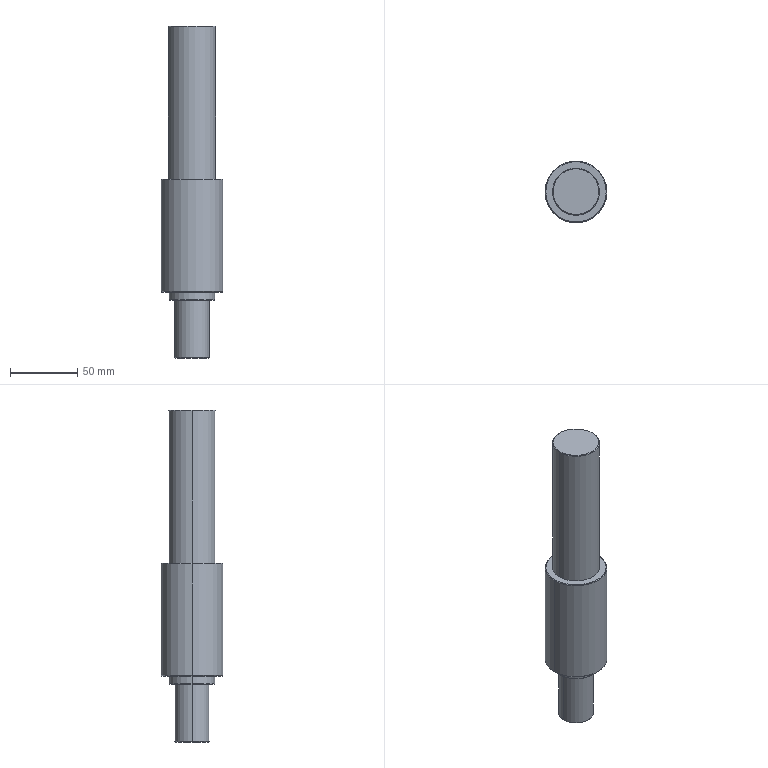Part | SolidWorks | features ICE 3, Chamfer 1, Extrusion 1 | 1 solid | 23 faces | box 46 x 46 x 247 mm | volume 277485 mm3 | cone 10 | cylinder 8 | plane 5 | commonest cylinder face diameters 26 x2 34 x2 35 x2 46 x2
STEP:
#1=CARTESIAN_POINT('',(17.,0.,57.));
#2=VERTEX_POINT('',#1);
#3=CARTESIAN_POINT('',(-17.,0.,57.));
#4=VERTEX_POINT('',#3);
#5=CARTESIAN_POINT('',(0.,0.,57.));
#6=DIRECTION('',(0.,0.,1.));
#7=DIRECTION('',(1.,0.,0.));
#8=AXIS2_PLACEMENT_3D('',#5,#6,#7);
#9=CIRCLE('',#8,17.);
#10=EDGE_CURVE('',#2,#4,#9,.T.);
#11=ORIENTED_EDGE('',*,*,#10,.F.);
#12=CARTESIAN_POINT('',(17.5,0.,56.5));
#13=VERTEX_POINT('',#12);
#14=CARTESIAN_POINT('',(17.,0.,57.));
#15=DIRECTION('',(0.7071,0.,-0.7071));
#16=VECTOR('',#15,1000.);
#17=LINE('',#14,#16);
#18=EDGE_CURVE('',#2,#13,#17,.T.);
#19=ORIENTED_EDGE('',*,*,#18,.T.);
#20=CARTESIAN_POINT('',(-17.5,0.,56.5));
#21=VERTEX_POINT('',#20);
#22=CARTESIAN_POINT('',(0.,0.,56.5));
#23=DIRECTION('',(0.,0.,-1.));
#24=DIRECTION('',(1.,0.,0.));
#25=AXIS2_PLACEMENT_3D('',#22,#23,#24);
#26=CIRCLE('',#25,17.5);
#27=EDGE_CURVE('',#21,#13,#26,.T.);
#28=ORIENTED_EDGE('',*,*,#27,.F.);
#29=CARTESIAN_POINT('',(-17.,0.,57.));
#30=DIRECTION('',(-0.7071,0.,-0.7071));
#31=VECTOR('',#30,1000.);
#32=LINE('',#29,#31);
#33=EDGE_CURVE('',#4,#21,#32,.T.);
#34=ORIENTED_EDGE('',*,*,#33,.F.);
#35=EDGE_LOOP('',(#11,#19,#28,#34));
#36=FACE_OUTER_BOUND('',#35,.T.);
#37=CARTESIAN_POINT('',(0.,0.,57.));
#38=DIRECTION('',(0.,0.,-1.));
#39=DIRECTION('',(-1.,0.,0.));
#40=AXIS2_PLACEMENT_3D('',#37,#38,#39);
#41=CONICAL_SURFACE('',#40,17.,0.7854);
#42=ADVANCED_FACE('',(#36),#41,.T.);
#43=CARTESIAN_POINT('',(22.5,0.,-57.));
#44=VERTEX_POINT('',#43);
#45=CARTESIAN_POINT('',(-22.5,0.,-57.));
#46=VERTEX_POINT('',#45);
#47=CARTESIAN_POINT('',(0.,0.,-57.));
#48=DIRECTION('',(0.,0.,1.));
#49=DIRECTION('',(-1.,0.,0.));
#50=AXIS2_PLACEMENT_3D('',#47,#48,#49);
#51=CIRCLE('',#50,22.5);
#52=EDGE_CURVE('',#44,#46,#51,.T.);
#53=ORIENTED_EDGE('',*,*,#52,.F.);
#54=CARTESIAN_POINT('',(23.,0.,-57.5));
#55=VERTEX_POINT('',#54);
#56=CARTESIAN_POINT('',(23.,0.,-57.5));
#57=DIRECTION('',(0.7071,0.,-0.7071));
#58=VECTOR('',#57,1000.);
#59=LINE('',#56,#58);
#60=EDGE_CURVE('',#44,#55,#59,.T.);
#61=ORIENTED_EDGE('',*,*,#60,.T.);
#62=CARTESIAN_POINT('',(-23.,0.,-57.5));
#63=VERTEX_POINT('',#62);
#64=CARTESIAN_POINT('',(0.,0.,-57.5));
#65=DIRECTION('',(0.,0.,-1.));
#66=DIRECTION('',(-1.,0.,0.));
#67=AXIS2_PLACEMENT_3D('',#64,#65,#66);
#68=CIRCLE('',#67,23.);
#69=EDGE_CURVE('',#63,#55,#68,.T.);
#70=ORIENTED_EDGE('',*,*,#69,.F.);
#71=CARTESIAN_POINT('',(-23.,0.,-57.5));
#72=DIRECTION('',(-0.7071,0.,-0.7071));
#73=VECTOR('',#72,1000.);
#74=LINE('',#71,#73);
#75=EDGE_CURVE('',#46,#63,#74,.T.);
#76=ORIENTED_EDGE('',*,*,#75,.F.);
#77=EDGE_LOOP('',(#53,#61,#70,#76));
#78=FACE_OUTER_BOUND('',#77,.T.);
#79=CARTESIAN_POINT('',(0.,0.,-57.5));
#80=DIRECTION('',(0.,0.,-1.));
#81=DIRECTION('',(-1.,0.,0.));
#82=AXIS2_PLACEMENT_3D('',#79,#80,#81);
#83=CONICAL_SURFACE('',#82,23.,0.7854);
#84=ADVANCED_FACE('',(#78),#83,.T.);
#85=CARTESIAN_POINT('',(-16.5,0.,-147.));
#86=VERTEX_POINT('',#85);
#87=CARTESIAN_POINT('',(16.5,0.,-147.));
#88=VERTEX_POINT('',#87);
#89=CARTESIAN_POINT('',(0.,0.,-147.));
#90=DIRECTION('',(0.,0.,-1.));
#91=DIRECTION('',(-1.,0.,0.));
#92=AXIS2_PLACEMENT_3D('',#89,#90,#91);
#93=CIRCLE('',#92,16.5);
#94=EDGE_CURVE('',#86,#88,#93,.T.);
#95=ORIENTED_EDGE('',*,*,#94,.F.);
#96=CARTESIAN_POINT('',(-17.,0.,-146.5));
#97=VERTEX_POINT('',#96);
#98=CARTESIAN_POINT('',(-16.5,0.,-147.));
#99=DIRECTION('',(-0.7071,0.,0.7071));
#100=VECTOR('',#99,1000.);
#101=LINE('',#98,#100);
#102=EDGE_CURVE('',#86,#97,#101,.T.);
#103=ORIENTED_EDGE('',*,*,#102,.T.);
#104=CARTESIAN_POINT('',(17.,0.,-146.5));
#105=VERTEX_POINT('',#104);
#106=CARTESIAN_POINT('',(0.,0.,-146.5));
#107=DIRECTION('',(0.,0.,1.));
#108=DIRECTION('',(-1.,0.,0.));
#109=AXIS2_PLACEMENT_3D('',#106,#107,#108);
#110=CIRCLE('',#109,17.);
#111=EDGE_CURVE('',#105,#97,#110,.T.);
#112=ORIENTED_EDGE('',*,*,#111,.F.);
#113=CARTESIAN_POINT('',(16.5,0.,-147.));
#114=DIRECTION('',(0.7071,0.,0.7071));
#115=VECTOR('',#114,1000.);
#116=LINE('',#113,#115);
#117=EDGE_CURVE('',#88,#105,#116,.T.);
#118=ORIENTED_EDGE('',*,*,#117,.F.);
#119=EDGE_LOOP('',(#95,#103,#112,#118));
#120=FACE_OUTER_BOUND('',#119,.T.);
#121=CARTESIAN_POINT('',(0.,0.,-147.));
#122=DIRECTION('',(0.,0.,1.));
#123=DIRECTION('',(1.,0.,0.));
#124=AXIS2_PLACEMENT_3D('',#121,#122,#123);
#125=CONICAL_SURFACE('',#124,16.5,0.7854);
#126=ADVANCED_FACE('',(#120),#125,.T.);
#127=CARTESIAN_POINT('',(-22.5,0.,-141.));
#128=VERTEX_POINT('',#127);
#129=CARTESIAN_POINT('',(22.5,0.,-141.));
#130=VERTEX_POINT('',#129);
#131=CARTESIAN_POINT('',(0.,0.,-141.));
#132=DIRECTION('',(0.,0.,-1.));
#133=DIRECTION('',(-1.,0.,0.));
#134=AXIS2_PLACEMENT_3D('',#131,#132,#133);
#135=CIRCLE('',#134,22.5);
#136=EDGE_CURVE('',#128,#130,#135,.T.);
#137=ORIENTED_EDGE('',*,*,#136,.F.);
#138=CARTESIAN_POINT('',(-23.,0.,-140.5));
#139=VERTEX_POINT('',#138);
#140=CARTESIAN_POINT('',(-22.5,0.,-141.));
#141=DIRECTION('',(-0.7071,0.,0.7071));
#142=VECTOR('',#141,1000.);
#143=LINE('',#140,#142);
#144=EDGE_CURVE('',#128,#139,#143,.T.);
#145=ORIENTED_EDGE('',*,*,#144,.T.);
#146=CARTESIAN_POINT('',(23.,0.,-140.5));
#147=VERTEX_POINT('',#146);
#148=CARTESIAN_POINT('',(0.,0.,-140.5));
#149=DIRECTION('',(0.,0.,1.));
#150=DIRECTION('',(-1.,0.,0.));
#151=AXIS2_PLACEMENT_3D('',#148,#149,#150);
#152=CIRCLE('',#151,23.);
#153=EDGE_CURVE('',#147,#139,#152,.T.);
#154=ORIENTED_EDGE('',*,*,#153,.F.);
#155=CARTESIAN_POINT('',(22.5,0.,-141.));
#156=DIRECTION('',(0.7071,0.,0.7071));
#157=VECTOR('',#156,1000.);
#158=LINE('',#155,#157);
#159=EDGE_CURVE('',#130,#147,#158,.T.);
#160=ORIENTED_EDGE('',*,*,#159,.F.);
#161=EDGE_LOOP('',(#137,#145,#154,#160));
#162=FACE_OUTER_BOUND('',#161,.T.);
#163=CARTESIAN_POINT('',(0.,0.,-141.));
#164=DIRECTION('',(0.,0.,1.));
#165=DIRECTION('',(1.,0.,0.));
#166=AXIS2_PLACEMENT_3D('',#163,#164,#165);
#167=CONICAL_SURFACE('',#166,22.5,0.7854);
#168=ADVANCED_FACE('',(#162),#167,.T.);
#169=CARTESIAN_POINT('',(-12.5,0.,-190.));
#170=VERTEX_POINT('',#169);
#171=CARTESIAN_POINT('',(12.5,0.,-190.));
#172=VERTEX_POINT('',#171);
#173=CARTESIAN_POINT('',(0.,0.,-190.));
#174=DIRECTION('',(0.,0.,-1.));
#175=DIRECTION('',(-1.,0.,0.));
#176=AXIS2_PLACEMENT_3D('',#173,#174,#175);
#177=CIRCLE('',#176,12.5);
#178=EDGE_CURVE('',#170,#172,#177,.T.);
#179=ORIENTED_EDGE('',*,*,#178,.F.);
#180=CARTESIAN_POINT('',(-13.,0.,-189.5));
#181=VERTEX_POINT('',#180);
#182=CARTESIAN_POINT('',(-12.5,0.,-190.));
#183=DIRECTION('',(-0.7071,0.,0.7071));
#184=VECTOR('',#183,1000.);
#185=LINE('',#182,#184);
#186=EDGE_CURVE('',#170,#181,#185,.T.);
#187=ORIENTED_EDGE('',*,*,#186,.T.);
#188=CARTESIAN_POINT('',(13.,0.,-189.5));
#189=VERTEX_POINT('',#188);
#190=CARTESIAN_POINT('',(0.,0.,-189.5));
#191=DIRECTION('',(0.,0.,1.));
#192=DIRECTION('',(-1.,0.,0.));
#193=AXIS2_PLACEMENT_3D('',#190,#191,#192);
#194=CIRCLE('',#193,13.);
#195=EDGE_CURVE('',#189,#181,#194,.T.);
#196=ORIENTED_EDGE('',*,*,#195,.F.);
#197=CARTESIAN_POINT('',(12.5,0.,-190.));
#198=DIRECTION('',(0.7071,0.,0.7071));
#199=VECTOR('',#198,1000.);
#200=LINE('',#197,#199);
#201=EDGE_CURVE('',#172,#189,#200,.T.);
#202=ORIENTED_EDGE('',*,*,#201,.F.);
#203=EDGE_LOOP('',(#179,#187,#196,#202));
#204=FACE_OUTER_BOUND('',#203,.T.);
#205=CARTESIAN_POINT('',(0.,0.,-190.));
#206=DIRECTION('',(0.,0.,1.));
#207=DIRECTION('',(1.,0.,0.));
#208=AXIS2_PLACEMENT_3D('',#205,#206,#207);
#209=CONICAL_SURFACE('',#208,12.5,0.7854);
#210=ADVANCED_FACE('',(#204),#209,.T.);
#211=ORIENTED_EDGE('',*,*,#195,.T.);
#212=CARTESIAN_POINT('',(-13.,0.,-147.));
#213=VERTEX_POINT('',#212);
#214=CARTESIAN_POINT('',(-13.,0.,-190.));
#215=DIRECTION('',(0.,0.,1.));
#216=VECTOR('',#215,1000.);
#217=LINE('',#214,#216);
#218=EDGE_CURVE('',#181,#213,#217,.T.);
#219=ORIENTED_EDGE('',*,*,#218,.T.);
#220=CARTESIAN_POINT('',(13.,0.,-147.));
#221=VERTEX_POINT('',#220);
#222=CARTESIAN_POINT('',(0.,0.,-147.));
#223=DIRECTION('',(0.,0.,-1.));
#224=DIRECTION('',(-1.,0.,0.));
#225=AXIS2_PLACEMENT_3D('',#222,#223,#224);
#226=CIRCLE('',#225,13.);
#227=EDGE_CURVE('',#213,#221,#226,.T.);
#228=ORIENTED_EDGE('',*,*,#227,.T.);
#229=CARTESIAN_POINT('',(13.,0.,-190.));
#230=DIRECTION('',(0.,0.,1.));
#231=VECTOR('',#230,1000.);
#232=LINE('',#229,#231);
#233=EDGE_CURVE('',#189,#221,#232,.T.);
#234=ORIENTED_EDGE('',*,*,#233,.F.);
#235=EDGE_LOOP('',(#211,#219,#228,#234));
#236=FACE_OUTER_BOUND('',#235,.T.);
#237=CARTESIAN_POINT('',(0.,0.,-190.));
#238=DIRECTION('',(0.,0.,1.));
#239=DIRECTION('',(1.,0.,0.));
#240=AXIS2_PLACEMENT_3D('',#237,#238,#239);
#241=CYLINDRICAL_SURFACE('',#240,13.);
#242=ADVANCED_FACE('',(#236),#241,.T.);
#243=ORIENTED_EDGE('',*,*,#111,.T.);
#244=CARTESIAN_POINT('',(-17.,0.,-141.));
#245=VERTEX_POINT('',#244);
#246=CARTESIAN_POINT('',(-17.,0.,-147.));
#247=DIRECTION('',(0.,0.,1.));
#248=VECTOR('',#247,1000.);
#249=LINE('',#246,#248);
#250=EDGE_CURVE('',#97,#245,#249,.T.);
#251=ORIENTED_EDGE('',*,*,#250,.T.);
#252=CARTESIAN_POINT('',(17.,0.,-141.));
#253=VERTEX_POINT('',#252);
#254=CARTESIAN_POINT('',(0.,0.,-141.));
#255=DIRECTION('',(0.,0.,-1.));
#256=DIRECTION('',(-1.,0.,0.));
#257=AXIS2_PLACEMENT_3D('',#254,#255,#256);
#258=CIRCLE('',#257,17.);
#259=EDGE_CURVE('',#245,#253,#258,.T.);
#260=ORIENTED_EDGE('',*,*,#259,.T.);
#261=CARTESIAN_POINT('',(17.,0.,-147.));
#262=DIRECTION('',(0.,0.,1.));
#263=VECTOR('',#262,1000.);
#264=LINE('',#261,#263);
#265=EDGE_CURVE('',#105,#253,#264,.T.);
#266=ORIENTED_EDGE('',*,*,#265,.F.);
#267=EDGE_LOOP('',(#243,#251,#260,#266));
#268=FACE_OUTER_BOUND('',#267,.T.);
#269=CARTESIAN_POINT('',(0.,0.,-147.));
#270=DIRECTION('',(0.,0.,1.));
#271=DIRECTION('',(1.,0.,0.));
#272=AXIS2_PLACEMENT_3D('',#269,#270,#271);
#273=CYLINDRICAL_SURFACE('',#272,17.);
#274=ADVANCED_FACE('',(#268),#273,.T.);
#275=ORIENTED_EDGE('',*,*,#153,.T.);
#276=CARTESIAN_POINT('',(-23.,0.,-141.));
#277=DIRECTION('',(0.,0.,1.));
#278=VECTOR('',#277,1000.);
#279=LINE('',#276,#278);
#280=EDGE_CURVE('',#139,#63,#279,.T.);
#281=ORIENTED_EDGE('',*,*,#280,.T.);
#282=ORIENTED_EDGE('',*,*,#69,.T.);
#283=CARTESIAN_POINT('',(23.,0.,-141.));
#284=DIRECTION('',(0.,0.,1.));
#285=VECTOR('',#284,1000.);
#286=LINE('',#283,#285);
#287=EDGE_CURVE('',#147,#55,#286,.T.);
#288=ORIENTED_EDGE('',*,*,#287,.F.);
#289=EDGE_LOOP('',(#275,#281,#282,#288));
#290=FACE_OUTER_BOUND('',#289,.T.);
#291=CARTESIAN_POINT('',(0.,0.,-141.));
#292=DIRECTION('',(0.,0.,1.));
#293=DIRECTION('',(1.,0.,0.));
#294=AXIS2_PLACEMENT_3D('',#291,#292,#293);
#295=CYLINDRICAL_SURFACE('',#294,23.);
#296=ADVANCED_FACE('',(#290),#295,.T.);
#297=ORIENTED_EDGE('',*,*,#27,.T.);
#298=CARTESIAN_POINT('',(17.5,0.,-57.));
#299=VERTEX_POINT('',#298);
#300=CARTESIAN_POINT('',(17.5,0.,57.));
#301=DIRECTION('',(0.,0.,-1.));
#302=VECTOR('',#301,1000.);
#303=LINE('',#300,#302);
#304=EDGE_CURVE('',#13,#299,#303,.T.);
#305=ORIENTED_EDGE('',*,*,#304,.T.);
#306=CARTESIAN_POINT('',(-17.5,0.,-57.));
#307=VERTEX_POINT('',#306);
#308=CARTESIAN_POINT('',(0.,0.,-57.));
#309=DIRECTION('',(0.,0.,-1.));
#310=DIRECTION('',(-1.,0.,0.));
#311=AXIS2_PLACEMENT_3D('',#308,#309,#310);
#312=CIRCLE('',#311,17.5);
#313=EDGE_CURVE('',#307,#299,#312,.T.);
#314=ORIENTED_EDGE('',*,*,#313,.F.);
#315=CARTESIAN_POINT('',(-17.5,0.,57.));
#316=DIRECTION('',(0.,0.,-1.));
#317=VECTOR('',#316,1000.);
#318=LINE('',#315,#317);
#319=EDGE_CURVE('',#21,#307,#318,.T.);
#320=ORIENTED_EDGE('',*,*,#319,.F.);
#321=EDGE_LOOP('',(#297,#305,#314,#320));
#322=FACE_OUTER_BOUND('',#321,.T.);
#323=CARTESIAN_POINT('',(0.,0.,57.));
#324=DIRECTION('',(0.,0.,-1.));
#325=DIRECTION('',(-1.,0.,0.));
#326=AXIS2_PLACEMENT_3D('',#323,#324,#325);
#327=CYLINDRICAL_SURFACE('',#326,17.5);
#328=ADVANCED_FACE('',(#322),#327,.T.);
#329=CARTESIAN_POINT('',(0.,0.,-147.));
#330=DIRECTION('',(0.,0.,-1.));
#331=DIRECTION('',(-1.,0.,0.));
#332=AXIS2_PLACEMENT_3D('',#329,#330,#331);
#333=CIRCLE('',#332,16.5);
#334=EDGE_CURVE('',#88,#86,#333,.T.);
#335=ORIENTED_EDGE('',*,*,#334,.T.);
#336=ORIENTED_EDGE('',*,*,#94,.T.);
#337=EDGE_LOOP('',(#335,#336));
#338=FACE_OUTER_BOUND('',#337,.T.);
#339=CARTESIAN_POINT('',(0.,0.,-147.));
#340=DIRECTION('',(0.,0.,-1.));
#341=DIRECTION('',(-1.,0.,0.));
#342=AXIS2_PLACEMENT_3D('',#339,#340,#341);
#343=CIRCLE('',#342,13.);
#344=EDGE_CURVE('',#221,#213,#343,.T.);
#345=ORIENTED_EDGE('',*,*,#344,.F.);
#346=ORIENTED_EDGE('',*,*,#227,.F.);
#347=EDGE_LOOP('',(#345,#346));
#348=FACE_BOUND('',#347,.T.);
#349=CARTESIAN_POINT('',(0.,0.,-147.));
#350=DIRECTION('',(0.,0.,-1.));
#351=DIRECTION('',(-1.,0.,0.));
#352=AXIS2_PLACEMENT_3D('',#349,#350,#351);
#353=PLANE('',#352);
#354=ADVANCED_FACE('',(#338,#348),#353,.T.);
#355=CARTESIAN_POINT('',(0.,0.,-141.));
#356=DIRECTION('',(0.,0.,-1.));
#357=DIRECTION('',(-1.,0.,0.));
#358=AXIS2_PLACEMENT_3D('',#355,#356,#357);
#359=CIRCLE('',#358,22.5);
#360=EDGE_CURVE('',#130,#128,#359,.T.);
#361=ORIENTED_EDGE('',*,*,#360,.T.);
#362=ORIENTED_EDGE('',*,*,#136,.T.);
#363=EDGE_LOOP('',(#361,#362));
#364=FACE_OUTER_BOUND('',#363,.T.);
#365=CARTESIAN_POINT('',(0.,0.,-141.));
#366=DIRECTION('',(0.,0.,-1.));
#367=DIRECTION('',(-1.,0.,0.));
#368=AXIS2_PLACEMENT_3D('',#365,#366,#367);
#369=CIRCLE('',#368,17.);
#370=EDGE_CURVE('',#253,#245,#369,.T.);
#371=ORIENTED_EDGE('',*,*,#370,.F.);
#372=ORIENTED_EDGE('',*,*,#259,.F.);
#373=EDGE_LOOP('',(#371,#372));
#374=FACE_BOUND('',#373,.T.);
#375=CARTESIAN_POINT('',(0.,0.,-141.));
#376=DIRECTION('',(0.,0.,-1.));
#377=DIRECTION('',(-1.,0.,0.));
#378=AXIS2_PLACEMENT_3D('',#375,#376,#377);
#379=PLANE('',#378);
#380=ADVANCED_FACE('',(#364,#374),#379,.T.);
#381=ORIENTED_EDGE('',*,*,#304,.F.);
#382=CARTESIAN_POINT('',(0.,0.,56.5));
#383=DIRECTION('',(0.,0.,-1.));
#384=DIRECTION('',(1.,0.,0.));
#385=AXIS2_PLACEMENT_3D('',#382,#383,#384);
#386=CIRCLE('',#385,17.5);
#387=EDGE_CURVE('',#13,#21,#386,.T.);
#388=ORIENTED_EDGE('',*,*,#387,.T.);
#389=ORIENTED_EDGE('',*,*,#319,.T.);
#390=CARTESIAN_POINT('',(0.,0.,-57.));
#391=DIRECTION('',(0.,0.,-1.));
#392=DIRECTION('',(-1.,0.,0.));
#393=AXIS2_PLACEMENT_3D('',#390,#391,#392);
#394=CIRCLE('',#393,17.5);
#395=EDGE_CURVE('',#299,#307,#394,.T.);
#396=ORIENTED_EDGE('',*,*,#395,.F.);
#397=EDGE_LOOP('',(#381,#388,#389,#396));
#398=FACE_OUTER_BOUND('',#397,.T.);
#399=CARTESIAN_POINT('',(0.,0.,57.));
#400=DIRECTION('',(0.,0.,-1.));
#401=DIRECTION('',(-1.,0.,0.));
#402=AXIS2_PLACEMENT_3D('',#399,#400,#401);
#403=CYLINDRICAL_SURFACE('',#402,17.5);
#404=ADVANCED_FACE('',(#398),#403,.T.);
#405=CARTESIAN_POINT('',(0.,0.,57.));
#406=DIRECTION('',(0.,0.,1.));
#407=DIRECTION('',(1.,0.,0.));
#408=AXIS2_PLACEMENT_3D('',#405,#406,#407);
#409=CIRCLE('',#408,17.);
#410=EDGE_CURVE('',#4,#2,#409,.T.);
#411=ORIENTED_EDGE('',*,*,#410,.T.);
#412=ORIENTED_EDGE('',*,*,#10,.T.);
#413=EDGE_LOOP('',(#411,#412));
#414=FACE_OUTER_BOUND('',#413,.T.);
#415=CARTESIAN_POINT('',(0.,0.,57.));
#416=DIRECTION('',(0.,0.,1.));
#417=DIRECTION('',(1.,0.,0.));
#418=AXIS2_PLACEMENT_3D('',#415,#416,#417);
#419=PLANE('',#418);
#420=ADVANCED_FACE('',(#414),#419,.T.);
#421=CARTESIAN_POINT('',(0.,0.,-57.));
#422=DIRECTION('',(0.,0.,1.));
#423=DIRECTION('',(-1.,0.,0.));
#424=AXIS2_PLACEMENT_3D('',#421,#422,#423);
#425=CIRCLE('',#424,22.5);
#426=EDGE_CURVE('',#46,#44,#425,.T.);
#427=ORIENTED_EDGE('',*,*,#426,.T.);
#428=ORIENTED_EDGE('',*,*,#52,.T.);
#429=EDGE_LOOP('',(#427,#428));
#430=FACE_OUTER_BOUND('',#429,.T.);
#431=ORIENTED_EDGE('',*,*,#313,.T.);
#432=ORIENTED_EDGE('',*,*,#395,.T.);
#433=EDGE_LOOP('',(#431,#432));
#434=FACE_BOUND('',#433,.T.);
#435=CARTESIAN_POINT('',(0.,0.,-57.));
#436=DIRECTION('',(0.,0.,-1.));
#437=DIRECTION('',(-1.,0.,0.));
#438=AXIS2_PLACEMENT_3D('',#435,#436,#437);
#439=PLANE('',#438);
#440=ADVANCED_FACE('',(#430,#434),#439,.F.);
#441=ORIENTED_EDGE('',*,*,#280,.F.);
#442=CARTESIAN_POINT('',(0.,0.,-140.5));
#443=DIRECTION('',(0.,0.,1.));
#444=DIRECTION('',(-1.,0.,0.));
#445=AXIS2_PLACEMENT_3D('',#442,#443,#444);
#446=CIRCLE('',#445,23.);
#447=EDGE_CURVE('',#139,#147,#446,.T.);
#448=ORIENTED_EDGE('',*,*,#447,.T.);
#449=ORIENTED_EDGE('',*,*,#287,.T.);
#450=CARTESIAN_POINT('',(0.,0.,-57.5));
#451=DIRECTION('',(0.,0.,-1.));
#452=DIRECTION('',(-1.,0.,0.));
#453=AXIS2_PLACEMENT_3D('',#450,#451,#452);
#454=CIRCLE('',#453,23.);
#455=EDGE_CURVE('',#55,#63,#454,.T.);
#456=ORIENTED_EDGE('',*,*,#455,.T.);
#457=EDGE_LOOP('',(#441,#448,#449,#456));
#458=FACE_OUTER_BOUND('',#457,.T.);
#459=CARTESIAN_POINT('',(0.,0.,-141.));
#460=DIRECTION('',(0.,0.,1.));
#461=DIRECTION('',(1.,0.,0.));
#462=AXIS2_PLACEMENT_3D('',#459,#460,#461);
#463=CYLINDRICAL_SURFACE('',#462,23.);
#464=ADVANCED_FACE('',(#458),#463,.T.);
#465=ORIENTED_EDGE('',*,*,#250,.F.);
#466=CARTESIAN_POINT('',(0.,0.,-146.5));
#467=DIRECTION('',(0.,0.,1.));
#468=DIRECTION('',(-1.,0.,0.));
#469=AXIS2_PLACEMENT_3D('',#466,#467,#468);
#470=CIRCLE('',#469,17.);
#471=EDGE_CURVE('',#97,#105,#470,.T.);
#472=ORIENTED_EDGE('',*,*,#471,.T.);
#473=ORIENTED_EDGE('',*,*,#265,.T.);
#474=ORIENTED_EDGE('',*,*,#370,.T.);
#475=EDGE_LOOP('',(#465,#472,#473,#474));
#476=FACE_OUTER_BOUND('',#475,.T.);
#477=CARTESIAN_POINT('',(0.,0.,-147.));
#478=DIRECTION('',(0.,0.,1.));
#479=DIRECTION('',(1.,0.,0.));
#480=AXIS2_PLACEMENT_3D('',#477,#478,#479);
#481=CYLINDRICAL_SURFACE('',#480,17.);
#482=ADVANCED_FACE('',(#476),#481,.T.);
#483=ORIENTED_EDGE('',*,*,#218,.F.);
#484=CARTESIAN_POINT('',(0.,0.,-189.5));
#485=DIRECTION('',(0.,0.,1.));
#486=DIRECTION('',(-1.,0.,0.));
#487=AXIS2_PLACEMENT_3D('',#484,#485,#486);
#488=CIRCLE('',#487,13.);
#489=EDGE_CURVE('',#181,#189,#488,.T.);
#490=ORIENTED_EDGE('',*,*,#489,.T.);
#491=ORIENTED_EDGE('',*,*,#233,.T.);
#492=ORIENTED_EDGE('',*,*,#344,.T.);
#493=EDGE_LOOP('',(#483,#490,#491,#492));
#494=FACE_OUTER_BOUND('',#493,.T.);
#495=CARTESIAN_POINT('',(0.,0.,-190.));
#496=DIRECTION('',(0.,0.,1.));
#497=DIRECTION('',(1.,0.,0.));
#498=AXIS2_PLACEMENT_3D('',#495,#496,#497);
#499=CYLINDRICAL_SURFACE('',#498,13.);
#500=ADVANCED_FACE('',(#494),#499,.T.);
#501=CARTESIAN_POINT('',(0.,0.,-190.));
#502=DIRECTION('',(0.,0.,-1.));
#503=DIRECTION('',(-1.,0.,0.));
#504=AXIS2_PLACEMENT_3D('',#501,#502,#503);
#505=CIRCLE('',#504,12.5);
#506=EDGE_CURVE('',#172,#170,#505,.T.);
#507=ORIENTED_EDGE('',*,*,#506,.T.);
#508=ORIENTED_EDGE('',*,*,#178,.T.);
#509=EDGE_LOOP('',(#507,#508));
#510=FACE_OUTER_BOUND('',#509,.T.);
#511=CARTESIAN_POINT('',(0.,0.,-190.));
#512=DIRECTION('',(0.,0.,-1.));
#513=DIRECTION('',(-1.,0.,0.));
#514=AXIS2_PLACEMENT_3D('',#511,#512,#513);
#515=PLANE('',#514);
#516=ADVANCED_FACE('',(#510),#515,.T.);
#517=ORIENTED_EDGE('',*,*,#186,.F.);
#518=ORIENTED_EDGE('',*,*,#506,.F.);
#519=ORIENTED_EDGE('',*,*,#201,.T.);
#520=ORIENTED_EDGE('',*,*,#489,.F.);
#521=EDGE_LOOP('',(#517,#518,#519,#520));
#522=FACE_OUTER_BOUND('',#521,.T.);
#523=CARTESIAN_POINT('',(0.,0.,-190.));
#524=DIRECTION('',(0.,0.,1.));
#525=DIRECTION('',(1.,0.,0.));
#526=AXIS2_PLACEMENT_3D('',#523,#524,#525);
#527=CONICAL_SURFACE('',#526,12.5,0.7854);
#528=ADVANCED_FACE('',(#522),#527,.T.);
#529=ORIENTED_EDGE('',*,*,#144,.F.);
#530=ORIENTED_EDGE('',*,*,#360,.F.);
#531=ORIENTED_EDGE('',*,*,#159,.T.);
#532=ORIENTED_EDGE('',*,*,#447,.F.);
#533=EDGE_LOOP('',(#529,#530,#531,#532));
#534=FACE_OUTER_BOUND('',#533,.T.);
#535=CARTESIAN_POINT('',(0.,0.,-141.));
#536=DIRECTION('',(0.,0.,1.));
#537=DIRECTION('',(1.,0.,0.));
#538=AXIS2_PLACEMENT_3D('',#535,#536,#537);
#539=CONICAL_SURFACE('',#538,22.5,0.7854);
#540=ADVANCED_FACE('',(#534),#539,.T.);
#541=ORIENTED_EDGE('',*,*,#102,.F.);
#542=ORIENTED_EDGE('',*,*,#334,.F.);
#543=ORIENTED_EDGE('',*,*,#117,.T.);
#544=ORIENTED_EDGE('',*,*,#471,.F.);
#545=EDGE_LOOP('',(#541,#542,#543,#544));
#546=FACE_OUTER_BOUND('',#545,.T.);
#547=CARTESIAN_POINT('',(0.,0.,-147.));
#548=DIRECTION('',(0.,0.,1.));
#549=DIRECTION('',(1.,0.,0.));
#550=AXIS2_PLACEMENT_3D('',#547,#548,#549);
#551=CONICAL_SURFACE('',#550,16.5,0.7854);
#552=ADVANCED_FACE('',(#546),#551,.T.);
#553=ORIENTED_EDGE('',*,*,#60,.F.);
#554=ORIENTED_EDGE('',*,*,#426,.F.);
#555=ORIENTED_EDGE('',*,*,#75,.T.);
#556=ORIENTED_EDGE('',*,*,#455,.F.);
#557=EDGE_LOOP('',(#553,#554,#555,#556));
#558=FACE_OUTER_BOUND('',#557,.T.);
#559=CARTESIAN_POINT('',(0.,0.,-57.5));
#560=DIRECTION('',(0.,0.,-1.));
#561=DIRECTION('',(-1.,0.,0.));
#562=AXIS2_PLACEMENT_3D('',#559,#560,#561);
#563=CONICAL_SURFACE('',#562,23.,0.7854);
#564=ADVANCED_FACE('',(#558),#563,.T.);
#565=ORIENTED_EDGE('',*,*,#18,.F.);
#566=ORIENTED_EDGE('',*,*,#410,.F.);
#567=ORIENTED_EDGE('',*,*,#33,.T.);
#568=ORIENTED_EDGE('',*,*,#387,.F.);
#569=EDGE_LOOP('',(#565,#566,#567,#568));
#570=FACE_OUTER_BOUND('',#569,.T.);
#571=CARTESIAN_POINT('',(0.,0.,57.));
#572=DIRECTION('',(0.,0.,-1.));
#573=DIRECTION('',(-1.,0.,0.));
#574=AXIS2_PLACEMENT_3D('',#571,#572,#573);
#575=CONICAL_SURFACE('',#574,17.,0.7854);
#576=ADVANCED_FACE('',(#570),#575,.T.);
#577=CLOSED_SHELL('',(#42,#84,#126,#168,#210,#242,#274,#296,#328,#354,#380,#404,#420,#440,#464,#482,#500,#516,#528,#540,#552,#564,#576));
#578=MANIFOLD_SOLID_BREP('',#577);
#579=CARTESIAN_POINT('',(0.,0.,0.));
#580=DIRECTION('',(0.,0.,1.));
#581=DIRECTION('',(1.,0.,0.));
#582=AXIS2_PLACEMENT_3D('',#579,#580,#581);
#583=(LENGTH_UNIT()NAMED_UNIT(*)SI_UNIT(.MILLI.,.METRE.));
#584=UNCERTAINTY_MEASURE_WITH_UNIT(LENGTH_MEASURE(0.00001),#583,'','');
#585=(NAMED_UNIT(*)PLANE_ANGLE_UNIT()SI_UNIT($,.RADIAN.));
#586=(NAMED_UNIT(*)SI_UNIT($,.STERADIAN.)SOLID_ANGLE_UNIT());
#587=(GEOMETRIC_REPRESENTATION_CONTEXT(3)GLOBAL_UNCERTAINTY_ASSIGNED_CONTEXT((#584))GLOBAL_UNIT_ASSIGNED_CONTEXT((#583,#585,#586))REPRESENTATION_CONTEXT('',''));
#588=ADVANCED_BREP_SHAPE_REPRESENTATION('',(#578,#582),#587);